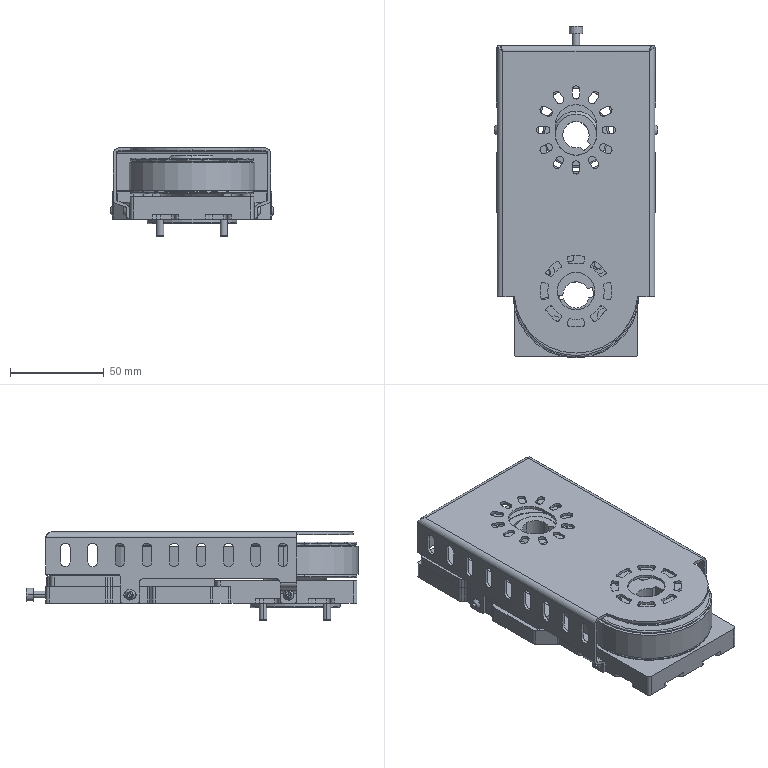Part | SolidWorks | features BaseBody 3, MoveFace 3, ICE 2 | 3 solids | 1559 faces | box 87.3 x 177.09 x 47 mm | volume 215586 mm3 | cylinder 887 | plane 588 | cone 50 | spline 34 | commonest cylinder face diameters 0.8 x249 2.98 x137 4 x108 63.7 x66 5 x54 2 x48